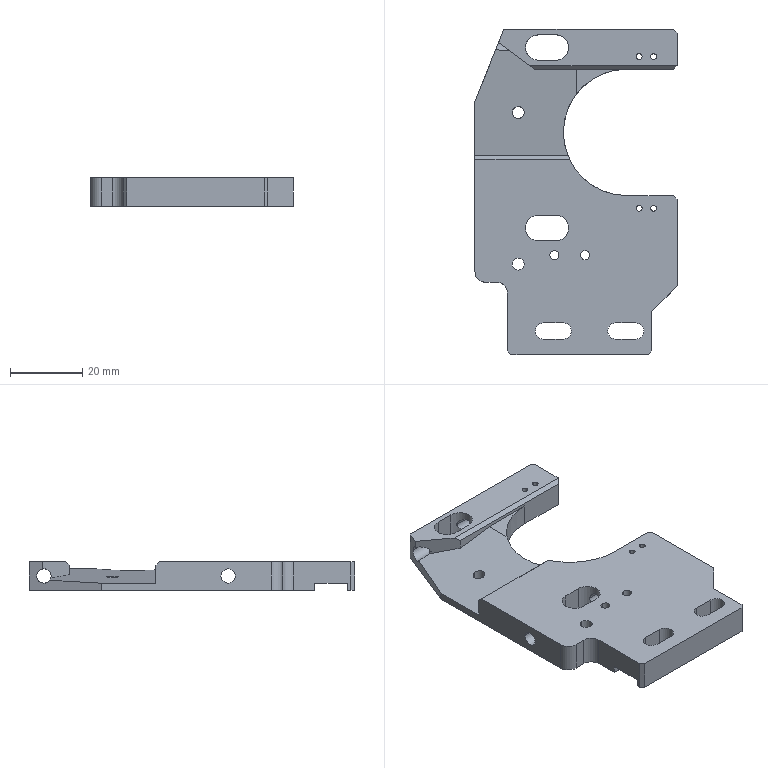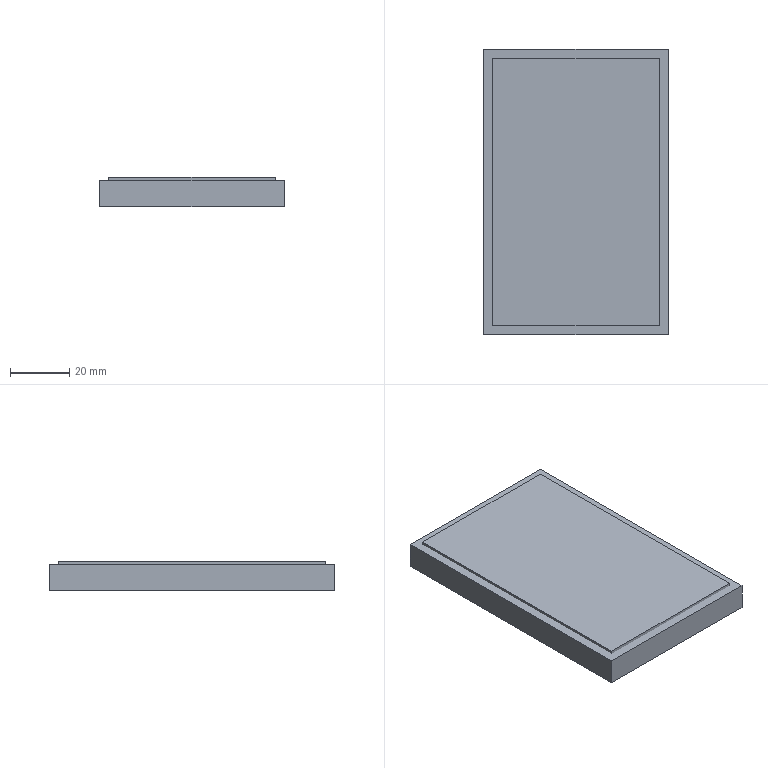CAM job | NX | 3-axis milling, drilling | part box 56 x 90 x 8 mm | stock box 62 x 96 x 10 mm
Tools:
number,name,description,diameter,corner_radius,flute_length,length,flutes
3,D63,Milling Tool-5 Parameters,63.0,0.0,50.0,75.0,2
1,D6A45,Milling Tool-5 Parameters,6.0,0.0,50.0,75.0,2
13,3.3ZT,Drilling Tool,3.3,0.0,35.0,50.0,2
22,2.5ZT,Drilling Tool,2.5,0.0,35.0,50.0,2
24,1.6ZT,Drilling Tool,1.6,0.0,35.0,50.0,2
4,D10,Milling Tool-5 Parameters,10.0,0.0,50.0,75.0,2
14,D10JING,Milling Tool-5 Parameters,10.0,0.0,50.0,75.0,2
16,D6,Milling Tool-5 Parameters,6.0,0.0,50.0,75.0,2
17,D4,Milling Tool-5 Parameters,4.0,0.0,50.0,75.0,2
7,D4R0.5,Milling Tool-5 Parameters,4.0,0.5,50.0,75.0,2
Operations:
program,operation,operation_type,tool,method,geometry_group,spindle_rpm,surface_speed,feed_per_tooth,feed_cut,feed_plunge,cut_length_mm,path_length_mm,cut_time_min,machine_time_min
1,FLOOR_WALL,VolumeBased25DMillingOperation,D63,METHOD,A,6500.0,1286.0,0.1154,1500.0,100.0,366.797,420.797,0.2445,0.2499
1,DRILLING,Operation,D6A45,METHOD,A,5000.0,94.0,0.025,250.0,0.0,32.0,273.964,0.128,0.1522
1,DRILLING_COPY,Operation,3.3ZT,METHOD,A,2000.0,21.0,0.0375,150.0,0.0,22.933,150.973,0.1529,0.1657
1,DRILLING_COPY_COPY,Operation,2.5ZT,METHOD,A,2000.0,21.0,0.0375,150.0,0.0,26.502,125.018,0.1767,0.1865
1,DRILLING_COPY_1_COPY,Operation,1.6ZT,METHOD,A,2000.0,37.0,0.0375,150.0,0.0,51.923,224.952,0.3462,0.3635
1,ADAPTIVE_MILLING,CavityMilling,D10,METHOD,A,7500.0,235.0,0.2,3000.0,1000.0,5233.076,5687.515,1.754,1.8
1,ZLEVEL_PROFILE,ZLevelMilling,D10JING,METHOD,A,7500.0,235.0,0.0667,1000.0,100.0,361.595,435.595,0.3616,0.369
1,CAVITY_MILL,CavityMilling,D6,METHOD,A,7500.0,141.0,0.12,1800.0,100.0,183.774,497.249,0.1021,0.1334
1,ZLEVEL_PROFILE_1_COPY_COPY,ZLevelMilling,D6,METHOD,A,7500.0,141.0,0.11,1650.0,1000.0,453.128,513.828,0.276,0.2821
1,ZLEVEL_PROFILE_1,ZLevelMilling,D4,METHOD,A,7500.0,94.0,0.1,1500.0,1000.0,879.406,1062.473,0.6105,0.6288
1,ZLEVEL_PROFILE_1_COPY,ZLevelMilling,D4,METHOD,A,7500.0,94.0,0.1,1500.0,1000.0,469.973,625.448,0.3375,0.3531
1,PLANAR_MILL,PlanarMilling,D6A45,METHOD,A,7500.0,141.0,0.0833,1250.0,100.0,506.152,1097.977,0.4049,0.4641
1,刀补16,ZLevelMilling,D6,METHOD,A,7500.0,141.0,0.0667,1000.0,1000.0,111.78,228.332,0.1118,0.1234
2,FLOOR_WALL_COPY,VolumeBased25DMillingOperation,D63,METHOD,B,6500.0,1286.0,0.1154,1500.0,100.0,697.594,834.391,0.4651,0.4787
2,CAVITY_MILL_COPY,CavityMilling,D6,METHOD,B,7500.0,141.0,0.12,1800.0,100.0,2295.236,2571.441,1.275,1.303
2,FIXED_CONTOUR,SurfaceContour,D4R0.5,METHOD,B,7500.0,94.0,0.1667,2500.0,1000.0,7425.555,7480.755,2.975,2.98
2,FIXED_CONTOUR_1,SurfaceContour,D4,METHOD,MCS_MILL_B,7500.0,94.0,0.0833,1250.0,100.0,54.974,115.774,0.044,0.0501
2,FIXED_CONTOUR_1_COPY_1,SurfaceContour,D4,METHOD,MCS_MILL_B,7500.0,94.0,0.0833,1250.0,100.0,42.431,104.831,0.0339,0.0402
2,PLANAR_MILL_COPY,PlanarMilling,D6A45,METHOD,B,7500.0,141.0,0.0833,1250.0,100.0,481.813,1198.047,0.3855,0.4571
2,PLANAR_MILL_COPY_COPY,PlanarMilling,D6A45,METHOD,B,7500.0,141.0,0.0833,1250.0,100.0,78.429,223.433,0.0627,0.0772